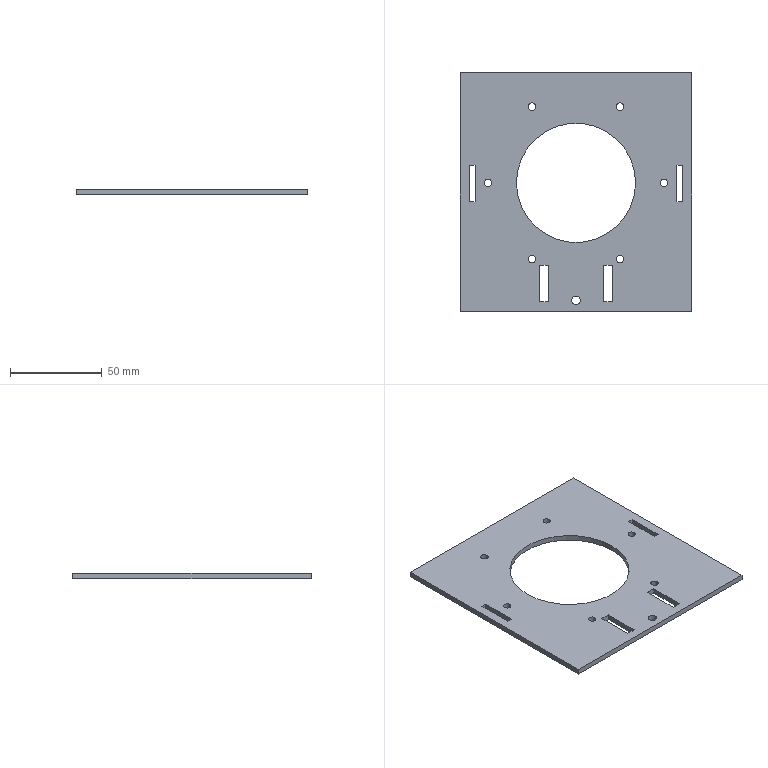Part | SolidWorks | features Cut 2, Extrusion 1, HoleWzd 1, MirrorPattern 1 | 1 solid | 38 faces | box 126 x 130 x 3 mm | volume 37973 mm3 | plane 22 | cylinder 16 | commonest cylinder face diameters 4 x12 4.6 x2 65 x2
STEP:
#1=CARTESIAN_POINT('',(-2.3,-64.,0.));
#2=VERTEX_POINT('',#1);
#3=CARTESIAN_POINT('',(2.3,-64.,0.));
#4=VERTEX_POINT('',#3);
#5=CARTESIAN_POINT('',(0.,-64.,0.));
#6=DIRECTION('',(0.,0.,1.));
#7=DIRECTION('',(1.,0.,0.));
#8=AXIS2_PLACEMENT_3D('',#5,#6,#7);
#9=CIRCLE('',#8,2.3);
#10=EDGE_CURVE('',#2,#4,#9,.T.);
#11=ORIENTED_EDGE('',*,*,#10,.F.);
#12=CARTESIAN_POINT('',(-2.3,-64.,3.));
#13=VERTEX_POINT('',#12);
#14=CARTESIAN_POINT('',(-2.3,-64.,0.));
#15=DIRECTION('',(0.,0.,1.));
#16=VECTOR('',#15,1000.);
#17=LINE('',#14,#16);
#18=EDGE_CURVE('',#2,#13,#17,.T.);
#19=ORIENTED_EDGE('',*,*,#18,.T.);
#20=CARTESIAN_POINT('',(2.3,-64.,3.));
#21=VERTEX_POINT('',#20);
#22=CARTESIAN_POINT('',(0.,-64.,3.));
#23=DIRECTION('',(0.,0.,1.));
#24=DIRECTION('',(1.,0.,0.));
#25=AXIS2_PLACEMENT_3D('',#22,#23,#24);
#26=CIRCLE('',#25,2.3);
#27=EDGE_CURVE('',#13,#21,#26,.T.);
#28=ORIENTED_EDGE('',*,*,#27,.T.);
#29=CARTESIAN_POINT('',(2.3,-64.,0.));
#30=DIRECTION('',(0.,0.,1.));
#31=VECTOR('',#30,1000.);
#32=LINE('',#29,#31);
#33=EDGE_CURVE('',#4,#21,#32,.T.);
#34=ORIENTED_EDGE('',*,*,#33,.F.);
#35=EDGE_LOOP('',(#11,#19,#28,#34));
#36=FACE_OUTER_BOUND('',#35,.T.);
#37=CARTESIAN_POINT('',(0.,-64.,0.));
#38=DIRECTION('',(0.,0.,1.));
#39=DIRECTION('',(1.,0.,0.));
#40=AXIS2_PLACEMENT_3D('',#37,#38,#39);
#41=CYLINDRICAL_SURFACE('',#40,2.3);
#42=ADVANCED_FACE('',(#36),#41,.F.);
#43=CARTESIAN_POINT('',(-26.,41.569,0.));
#44=VERTEX_POINT('',#43);
#45=CARTESIAN_POINT('',(-22.,41.569,0.));
#46=VERTEX_POINT('',#45);
#47=CARTESIAN_POINT('',(-24.,41.569,0.));
#48=DIRECTION('',(0.,0.,1.));
#49=DIRECTION('',(1.,0.,0.));
#50=AXIS2_PLACEMENT_3D('',#47,#48,#49);
#51=CIRCLE('',#50,2.);
#52=EDGE_CURVE('',#44,#46,#51,.T.);
#53=ORIENTED_EDGE('',*,*,#52,.F.);
#54=CARTESIAN_POINT('',(-26.,41.569,3.));
#55=VERTEX_POINT('',#54);
#56=CARTESIAN_POINT('',(-26.,41.569,3.));
#57=DIRECTION('',(0.,0.,1.));
#58=VECTOR('',#57,1000.);
#59=LINE('',#56,#58);
#60=EDGE_CURVE('',#44,#55,#59,.T.);
#61=ORIENTED_EDGE('',*,*,#60,.T.);
#62=CARTESIAN_POINT('',(-22.,41.569,3.));
#63=VERTEX_POINT('',#62);
#64=CARTESIAN_POINT('',(-24.,41.569,3.));
#65=DIRECTION('',(0.,0.,1.));
#66=DIRECTION('',(1.,0.,0.));
#67=AXIS2_PLACEMENT_3D('',#64,#65,#66);
#68=CIRCLE('',#67,2.);
#69=EDGE_CURVE('',#55,#63,#68,.T.);
#70=ORIENTED_EDGE('',*,*,#69,.T.);
#71=CARTESIAN_POINT('',(-22.,41.569,3.));
#72=DIRECTION('',(0.,0.,1.));
#73=VECTOR('',#72,1000.);
#74=LINE('',#71,#73);
#75=EDGE_CURVE('',#46,#63,#74,.T.);
#76=ORIENTED_EDGE('',*,*,#75,.F.);
#77=EDGE_LOOP('',(#53,#61,#70,#76));
#78=FACE_OUTER_BOUND('',#77,.T.);
#79=CARTESIAN_POINT('',(-24.,41.569,3.));
#80=DIRECTION('',(0.,0.,1.));
#81=DIRECTION('',(1.,0.,0.));
#82=AXIS2_PLACEMENT_3D('',#79,#80,#81);
#83=CYLINDRICAL_SURFACE('',#82,2.);
#84=ADVANCED_FACE('',(#78),#83,.F.);
#85=CARTESIAN_POINT('',(46.,0.,0.));
#86=VERTEX_POINT('',#85);
#87=CARTESIAN_POINT('',(50.,0.,0.));
#88=VERTEX_POINT('',#87);
#89=CARTESIAN_POINT('',(48.,0.,0.));
#90=DIRECTION('',(0.,0.,1.));
#91=DIRECTION('',(1.,0.,0.));
#92=AXIS2_PLACEMENT_3D('',#89,#90,#91);
#93=CIRCLE('',#92,2.);
#94=EDGE_CURVE('',#86,#88,#93,.T.);
#95=ORIENTED_EDGE('',*,*,#94,.F.);
#96=CARTESIAN_POINT('',(46.,0.,3.));
#97=VERTEX_POINT('',#96);
#98=CARTESIAN_POINT('',(46.,0.,3.));
#99=DIRECTION('',(0.,0.,1.));
#100=VECTOR('',#99,1000.);
#101=LINE('',#98,#100);
#102=EDGE_CURVE('',#86,#97,#101,.T.);
#103=ORIENTED_EDGE('',*,*,#102,.T.);
#104=CARTESIAN_POINT('',(50.,0.,3.));
#105=VERTEX_POINT('',#104);
#106=CARTESIAN_POINT('',(48.,0.,3.));
#107=DIRECTION('',(0.,0.,1.));
#108=DIRECTION('',(1.,0.,0.));
#109=AXIS2_PLACEMENT_3D('',#106,#107,#108);
#110=CIRCLE('',#109,2.);
#111=EDGE_CURVE('',#97,#105,#110,.T.);
#112=ORIENTED_EDGE('',*,*,#111,.T.);
#113=CARTESIAN_POINT('',(50.,0.,3.));
#114=DIRECTION('',(0.,0.,1.));
#115=VECTOR('',#114,1000.);
#116=LINE('',#113,#115);
#117=EDGE_CURVE('',#88,#105,#116,.T.);
#118=ORIENTED_EDGE('',*,*,#117,.F.);
#119=EDGE_LOOP('',(#95,#103,#112,#118));
#120=FACE_OUTER_BOUND('',#119,.T.);
#121=CARTESIAN_POINT('',(48.,0.,3.));
#122=DIRECTION('',(0.,0.,1.));
#123=DIRECTION('',(1.,0.,0.));
#124=AXIS2_PLACEMENT_3D('',#121,#122,#123);
#125=CYLINDRICAL_SURFACE('',#124,2.);
#126=ADVANCED_FACE('',(#120),#125,.F.);
#127=CARTESIAN_POINT('',(22.,41.569,0.));
#128=VERTEX_POINT('',#127);
#129=CARTESIAN_POINT('',(26.,41.569,0.));
#130=VERTEX_POINT('',#129);
#131=CARTESIAN_POINT('',(24.,41.569,0.));
#132=DIRECTION('',(0.,0.,1.));
#133=DIRECTION('',(1.,0.,0.));
#134=AXIS2_PLACEMENT_3D('',#131,#132,#133);
#135=CIRCLE('',#134,2.);
#136=EDGE_CURVE('',#128,#130,#135,.T.);
#137=ORIENTED_EDGE('',*,*,#136,.F.);
#138=CARTESIAN_POINT('',(22.,41.569,3.));
#139=VERTEX_POINT('',#138);
#140=CARTESIAN_POINT('',(22.,41.569,3.));
#141=DIRECTION('',(0.,0.,1.));
#142=VECTOR('',#141,1000.);
#143=LINE('',#140,#142);
#144=EDGE_CURVE('',#128,#139,#143,.T.);
#145=ORIENTED_EDGE('',*,*,#144,.T.);
#146=CARTESIAN_POINT('',(26.,41.569,3.));
#147=VERTEX_POINT('',#146);
#148=CARTESIAN_POINT('',(24.,41.569,3.));
#149=DIRECTION('',(0.,0.,1.));
#150=DIRECTION('',(1.,0.,0.));
#151=AXIS2_PLACEMENT_3D('',#148,#149,#150);
#152=CIRCLE('',#151,2.);
#153=EDGE_CURVE('',#139,#147,#152,.T.);
#154=ORIENTED_EDGE('',*,*,#153,.T.);
#155=CARTESIAN_POINT('',(26.,41.569,3.));
#156=DIRECTION('',(0.,0.,1.));
#157=VECTOR('',#156,1000.);
#158=LINE('',#155,#157);
#159=EDGE_CURVE('',#130,#147,#158,.T.);
#160=ORIENTED_EDGE('',*,*,#159,.F.);
#161=EDGE_LOOP('',(#137,#145,#154,#160));
#162=FACE_OUTER_BOUND('',#161,.T.);
#163=CARTESIAN_POINT('',(24.,41.569,3.));
#164=DIRECTION('',(0.,0.,1.));
#165=DIRECTION('',(1.,0.,0.));
#166=AXIS2_PLACEMENT_3D('',#163,#164,#165);
#167=CYLINDRICAL_SURFACE('',#166,2.);
#168=ADVANCED_FACE('',(#162),#167,.F.);
#169=CARTESIAN_POINT('',(22.,-41.569,0.));
#170=VERTEX_POINT('',#169);
#171=CARTESIAN_POINT('',(26.,-41.569,0.));
#172=VERTEX_POINT('',#171);
#173=CARTESIAN_POINT('',(24.,-41.569,0.));
#174=DIRECTION('',(0.,0.,1.));
#175=DIRECTION('',(1.,0.,0.));
#176=AXIS2_PLACEMENT_3D('',#173,#174,#175);
#177=CIRCLE('',#176,2.);
#178=EDGE_CURVE('',#170,#172,#177,.T.);
#179=ORIENTED_EDGE('',*,*,#178,.F.);
#180=CARTESIAN_POINT('',(22.,-41.569,3.));
#181=VERTEX_POINT('',#180);
#182=CARTESIAN_POINT('',(22.,-41.569,3.));
#183=DIRECTION('',(0.,0.,1.));
#184=VECTOR('',#183,1000.);
#185=LINE('',#182,#184);
#186=EDGE_CURVE('',#170,#181,#185,.T.);
#187=ORIENTED_EDGE('',*,*,#186,.T.);
#188=CARTESIAN_POINT('',(26.,-41.569,3.));
#189=VERTEX_POINT('',#188);
#190=CARTESIAN_POINT('',(24.,-41.569,3.));
#191=DIRECTION('',(0.,0.,1.));
#192=DIRECTION('',(1.,0.,0.));
#193=AXIS2_PLACEMENT_3D('',#190,#191,#192);
#194=CIRCLE('',#193,2.);
#195=EDGE_CURVE('',#181,#189,#194,.T.);
#196=ORIENTED_EDGE('',*,*,#195,.T.);
#197=CARTESIAN_POINT('',(26.,-41.569,3.));
#198=DIRECTION('',(0.,0.,1.));
#199=VECTOR('',#198,1000.);
#200=LINE('',#197,#199);
#201=EDGE_CURVE('',#172,#189,#200,.T.);
#202=ORIENTED_EDGE('',*,*,#201,.F.);
#203=EDGE_LOOP('',(#179,#187,#196,#202));
#204=FACE_OUTER_BOUND('',#203,.T.);
#205=CARTESIAN_POINT('',(24.,-41.569,3.));
#206=DIRECTION('',(0.,0.,1.));
#207=DIRECTION('',(1.,0.,0.));
#208=AXIS2_PLACEMENT_3D('',#205,#206,#207);
#209=CYLINDRICAL_SURFACE('',#208,2.);
#210=ADVANCED_FACE('',(#204),#209,.F.);
#211=CARTESIAN_POINT('',(-26.,-41.569,0.));
#212=VERTEX_POINT('',#211);
#213=CARTESIAN_POINT('',(-22.,-41.569,0.));
#214=VERTEX_POINT('',#213);
#215=CARTESIAN_POINT('',(-24.,-41.569,0.));
#216=DIRECTION('',(0.,0.,1.));
#217=DIRECTION('',(1.,0.,0.));
#218=AXIS2_PLACEMENT_3D('',#215,#216,#217);
#219=CIRCLE('',#218,2.);
#220=EDGE_CURVE('',#212,#214,#219,.T.);
#221=ORIENTED_EDGE('',*,*,#220,.F.);
#222=CARTESIAN_POINT('',(-26.,-41.569,3.));
#223=VERTEX_POINT('',#222);
#224=CARTESIAN_POINT('',(-26.,-41.569,3.));
#225=DIRECTION('',(0.,0.,1.));
#226=VECTOR('',#225,1000.);
#227=LINE('',#224,#226);
#228=EDGE_CURVE('',#212,#223,#227,.T.);
#229=ORIENTED_EDGE('',*,*,#228,.T.);
#230=CARTESIAN_POINT('',(-22.,-41.569,3.));
#231=VERTEX_POINT('',#230);
#232=CARTESIAN_POINT('',(-24.,-41.569,3.));
#233=DIRECTION('',(0.,0.,1.));
#234=DIRECTION('',(1.,0.,0.));
#235=AXIS2_PLACEMENT_3D('',#232,#233,#234);
#236=CIRCLE('',#235,2.);
#237=EDGE_CURVE('',#223,#231,#236,.T.);
#238=ORIENTED_EDGE('',*,*,#237,.T.);
#239=CARTESIAN_POINT('',(-22.,-41.569,3.));
#240=DIRECTION('',(0.,0.,1.));
#241=VECTOR('',#240,1000.);
#242=LINE('',#239,#241);
#243=EDGE_CURVE('',#214,#231,#242,.T.);
#244=ORIENTED_EDGE('',*,*,#243,.F.);
#245=EDGE_LOOP('',(#221,#229,#238,#244));
#246=FACE_OUTER_BOUND('',#245,.T.);
#247=CARTESIAN_POINT('',(-24.,-41.569,3.));
#248=DIRECTION('',(0.,0.,1.));
#249=DIRECTION('',(1.,0.,0.));
#250=AXIS2_PLACEMENT_3D('',#247,#248,#249);
#251=CYLINDRICAL_SURFACE('',#250,2.);
#252=ADVANCED_FACE('',(#246),#251,.F.);
#253=CARTESIAN_POINT('',(-50.,0.,0.));
#254=VERTEX_POINT('',#253);
#255=CARTESIAN_POINT('',(-46.,0.,0.));
#256=VERTEX_POINT('',#255);
#257=CARTESIAN_POINT('',(-48.,0.,0.));
#258=DIRECTION('',(0.,0.,1.));
#259=DIRECTION('',(1.,0.,0.));
#260=AXIS2_PLACEMENT_3D('',#257,#258,#259);
#261=CIRCLE('',#260,2.);
#262=EDGE_CURVE('',#254,#256,#261,.T.);
#263=ORIENTED_EDGE('',*,*,#262,.F.);
#264=CARTESIAN_POINT('',(-50.,0.,3.));
#265=VERTEX_POINT('',#264);
#266=CARTESIAN_POINT('',(-50.,0.,3.));
#267=DIRECTION('',(0.,0.,1.));
#268=VECTOR('',#267,1000.);
#269=LINE('',#266,#268);
#270=EDGE_CURVE('',#254,#265,#269,.T.);
#271=ORIENTED_EDGE('',*,*,#270,.T.);
#272=CARTESIAN_POINT('',(-46.,0.,3.));
#273=VERTEX_POINT('',#272);
#274=CARTESIAN_POINT('',(-48.,0.,3.));
#275=DIRECTION('',(0.,0.,1.));
#276=DIRECTION('',(1.,0.,0.));
#277=AXIS2_PLACEMENT_3D('',#274,#275,#276);
#278=CIRCLE('',#277,2.);
#279=EDGE_CURVE('',#265,#273,#278,.T.);
#280=ORIENTED_EDGE('',*,*,#279,.T.);
#281=CARTESIAN_POINT('',(-46.,0.,3.));
#282=DIRECTION('',(0.,0.,1.));
#283=VECTOR('',#282,1000.);
#284=LINE('',#281,#283);
#285=EDGE_CURVE('',#256,#273,#284,.T.);
#286=ORIENTED_EDGE('',*,*,#285,.F.);
#287=EDGE_LOOP('',(#263,#271,#280,#286));
#288=FACE_OUTER_BOUND('',#287,.T.);
#289=CARTESIAN_POINT('',(-48.,0.,3.));
#290=DIRECTION('',(0.,0.,1.));
#291=DIRECTION('',(1.,0.,0.));
#292=AXIS2_PLACEMENT_3D('',#289,#290,#291);
#293=CYLINDRICAL_SURFACE('',#292,2.);
#294=ADVANCED_FACE('',(#288),#293,.F.);
#295=CARTESIAN_POINT('',(-32.5,0.,3.));
#296=VERTEX_POINT('',#295);
#297=CARTESIAN_POINT('',(32.5,0.,3.));
#298=VERTEX_POINT('',#297);
#299=CARTESIAN_POINT('',(0.,0.,3.));
#300=DIRECTION('',(0.,0.,1.));
#301=DIRECTION('',(1.,0.,0.));
#302=AXIS2_PLACEMENT_3D('',#299,#300,#301);
#303=CIRCLE('',#302,32.5);
#304=EDGE_CURVE('',#296,#298,#303,.T.);
#305=ORIENTED_EDGE('',*,*,#304,.T.);
#306=CARTESIAN_POINT('',(32.5,0.,0.));
#307=VERTEX_POINT('',#306);
#308=CARTESIAN_POINT('',(32.5,0.,3.));
#309=DIRECTION('',(0.,0.,-1.));
#310=VECTOR('',#309,1000.);
#311=LINE('',#308,#310);
#312=EDGE_CURVE('',#298,#307,#311,.T.);
#313=ORIENTED_EDGE('',*,*,#312,.T.);
#314=CARTESIAN_POINT('',(-32.5,0.,0.));
#315=VERTEX_POINT('',#314);
#316=CARTESIAN_POINT('',(0.,0.,0.));
#317=DIRECTION('',(0.,0.,1.));
#318=DIRECTION('',(1.,0.,0.));
#319=AXIS2_PLACEMENT_3D('',#316,#317,#318);
#320=CIRCLE('',#319,32.5);
#321=EDGE_CURVE('',#315,#307,#320,.T.);
#322=ORIENTED_EDGE('',*,*,#321,.F.);
#323=CARTESIAN_POINT('',(-32.5,0.,3.));
#324=DIRECTION('',(0.,0.,-1.));
#325=VECTOR('',#324,1000.);
#326=LINE('',#323,#325);
#327=EDGE_CURVE('',#296,#315,#326,.T.);
#328=ORIENTED_EDGE('',*,*,#327,.F.);
#329=EDGE_LOOP('',(#305,#313,#322,#328));
#330=FACE_OUTER_BOUND('',#329,.T.);
#331=CARTESIAN_POINT('',(0.,0.,3.));
#332=DIRECTION('',(0.,0.,-1.));
#333=DIRECTION('',(-1.,0.,0.));
#334=AXIS2_PLACEMENT_3D('',#331,#332,#333);
#335=CYLINDRICAL_SURFACE('',#334,32.5);
#336=ADVANCED_FACE('',(#330),#335,.F.);
#337=CARTESIAN_POINT('',(0.,-64.,3.));
#338=DIRECTION('',(0.,0.,1.));
#339=DIRECTION('',(1.,0.,0.));
#340=AXIS2_PLACEMENT_3D('',#337,#338,#339);
#341=CIRCLE('',#340,2.3);
#342=EDGE_CURVE('',#21,#13,#341,.T.);
#343=ORIENTED_EDGE('',*,*,#342,.F.);
#344=ORIENTED_EDGE('',*,*,#27,.F.);
#345=EDGE_LOOP('',(#343,#344));
#346=FACE_BOUND('',#345,.T.);
#347=CARTESIAN_POINT('',(-24.,41.569,3.));
#348=DIRECTION('',(0.,0.,1.));
#349=DIRECTION('',(1.,0.,0.));
#350=AXIS2_PLACEMENT_3D('',#347,#348,#349);
#351=CIRCLE('',#350,2.);
#352=EDGE_CURVE('',#63,#55,#351,.T.);
#353=ORIENTED_EDGE('',*,*,#352,.F.);
#354=ORIENTED_EDGE('',*,*,#69,.F.);
#355=EDGE_LOOP('',(#353,#354));
#356=FACE_BOUND('',#355,.T.);
#357=CARTESIAN_POINT('',(48.,0.,3.));
#358=DIRECTION('',(0.,0.,1.));
#359=DIRECTION('',(1.,0.,0.));
#360=AXIS2_PLACEMENT_3D('',#357,#358,#359);
#361=CIRCLE('',#360,2.);
#362=EDGE_CURVE('',#105,#97,#361,.T.);
#363=ORIENTED_EDGE('',*,*,#362,.F.);
#364=ORIENTED_EDGE('',*,*,#111,.F.);
#365=EDGE_LOOP('',(#363,#364));
#366=FACE_BOUND('',#365,.T.);
#367=CARTESIAN_POINT('',(24.,41.569,3.));
#368=DIRECTION('',(0.,0.,1.));
#369=DIRECTION('',(1.,0.,0.));
#370=AXIS2_PLACEMENT_3D('',#367,#368,#369);
#371=CIRCLE('',#370,2.);
#372=EDGE_CURVE('',#147,#139,#371,.T.);
#373=ORIENTED_EDGE('',*,*,#372,.F.);
#374=ORIENTED_EDGE('',*,*,#153,.F.);
#375=EDGE_LOOP('',(#373,#374));
#376=FACE_BOUND('',#375,.T.);
#377=CARTESIAN_POINT('',(24.,-41.569,3.));
#378=DIRECTION('',(0.,0.,1.));
#379=DIRECTION('',(1.,0.,0.));
#380=AXIS2_PLACEMENT_3D('',#377,#378,#379);
#381=CIRCLE('',#380,2.);
#382=EDGE_CURVE('',#189,#181,#381,.T.);
#383=ORIENTED_EDGE('',*,*,#382,.F.);
#384=ORIENTED_EDGE('',*,*,#195,.F.);
#385=EDGE_LOOP('',(#383,#384));
#386=FACE_BOUND('',#385,.T.);
#387=CARTESIAN_POINT('',(-24.,-41.569,3.));
#388=DIRECTION('',(0.,0.,1.));
#389=DIRECTION('',(1.,0.,0.));
#390=AXIS2_PLACEMENT_3D('',#387,#388,#389);
#391=CIRCLE('',#390,2.);
#392=EDGE_CURVE('',#231,#223,#391,.T.);
#393=ORIENTED_EDGE('',*,*,#392,.F.);
#394=ORIENTED_EDGE('',*,*,#237,.F.);
#395=EDGE_LOOP('',(#393,#394));
#396=FACE_BOUND('',#395,.T.);
#397=CARTESIAN_POINT('',(-48.,0.,3.));
#398=DIRECTION('',(0.,0.,1.));
#399=DIRECTION('',(1.,0.,0.));
#400=AXIS2_PLACEMENT_3D('',#397,#398,#399);
#401=CIRCLE('',#400,2.);
#402=EDGE_CURVE('',#273,#265,#401,.T.);
#403=ORIENTED_EDGE('',*,*,#402,.F.);
#404=ORIENTED_EDGE('',*,*,#279,.F.);
#405=EDGE_LOOP('',(#403,#404));
#406=FACE_BOUND('',#405,.T.);
#407=CARTESIAN_POINT('',(15.05,-44.9,3.));
#408=VERTEX_POINT('',#407);
#409=CARTESIAN_POINT('',(15.05,-64.9,3.));
#410=VERTEX_POINT('',#409);
#411=CARTESIAN_POINT('',(15.05,-44.9,3.));
#412=DIRECTION('',(0.,-1.,0.));
#413=VECTOR('',#412,1000.);
#414=LINE('',#411,#413);
#415=EDGE_CURVE('',#408,#410,#414,.T.);
#416=ORIENTED_EDGE('',*,*,#415,.F.);
#417=CARTESIAN_POINT('',(19.95,-44.9,3.));
#418=VERTEX_POINT('',#417);
#419=CARTESIAN_POINT('',(19.95,-44.9,3.));
#420=DIRECTION('',(-1.,0.,0.));
#421=VECTOR('',#420,1000.);
#422=LINE('',#419,#421);
#423=EDGE_CURVE('',#418,#408,#422,.T.);
#424=ORIENTED_EDGE('',*,*,#423,.F.);
#425=CARTESIAN_POINT('',(19.95,-64.9,3.));
#426=VERTEX_POINT('',#425);
#427=CARTESIAN_POINT('',(19.95,-44.9,3.));
#428=DIRECTION('',(0.,1.,0.));
#429=VECTOR('',#428,1000.);
#430=LINE('',#427,#429);
#431=EDGE_CURVE('',#426,#418,#430,.T.);
#432=ORIENTED_EDGE('',*,*,#431,.F.);
#433=CARTESIAN_POINT('',(19.95,-64.9,3.));
#434=DIRECTION('',(1.,0.,0.));
#435=VECTOR('',#434,1000.);
#436=LINE('',#433,#435);
#437=EDGE_CURVE('',#410,#426,#436,.T.);
#438=ORIENTED_EDGE('',*,*,#437,.F.);
#439=EDGE_LOOP('',(#416,#424,#432,#438));
#440=FACE_BOUND('',#439,.T.);
#441=ORIENTED_EDGE('',*,*,#304,.F.);
#442=CARTESIAN_POINT('',(0.,0.,3.));
#443=DIRECTION('',(0.,0.,1.));
#444=DIRECTION('',(1.,0.,0.));
#445=AXIS2_PLACEMENT_3D('',#442,#443,#444);
#446=CIRCLE('',#445,32.5);
#447=EDGE_CURVE('',#298,#296,#446,.T.);
#448=ORIENTED_EDGE('',*,*,#447,.F.);
#449=EDGE_LOOP('',(#441,#448));
#450=FACE_BOUND('',#449,.T.);
#451=CARTESIAN_POINT('',(-63.,60.,3.));
#452=VERTEX_POINT('',#451);
#453=CARTESIAN_POINT('',(-63.,-70.,3.));
#454=VERTEX_POINT('',#453);
#455=CARTESIAN_POINT('',(-63.,60.,3.));
#456=DIRECTION('',(0.,-1.,0.));
#457=VECTOR('',#456,1000.);
#458=LINE('',#455,#457);
#459=EDGE_CURVE('',#452,#454,#458,.T.);
#460=ORIENTED_EDGE('',*,*,#459,.T.);
#461=CARTESIAN_POINT('',(63.,-70.,3.));
#462=VERTEX_POINT('',#461);
#463=CARTESIAN_POINT('',(-63.,-70.,3.));
#464=DIRECTION('',(1.,0.,0.));
#465=VECTOR('',#464,1000.);
#466=LINE('',#463,#465);
#467=EDGE_CURVE('',#454,#462,#466,.T.);
#468=ORIENTED_EDGE('',*,*,#467,.T.);
#469=CARTESIAN_POINT('',(63.,60.,3.));
#470=VERTEX_POINT('',#469);
#471=CARTESIAN_POINT('',(63.,60.,3.));
#472=DIRECTION('',(0.,1.,0.));
#473=VECTOR('',#472,1000.);
#474=LINE('',#471,#473);
#475=EDGE_CURVE('',#462,#470,#474,.T.);
#476=ORIENTED_EDGE('',*,*,#475,.T.);
#477=CARTESIAN_POINT('',(-63.,60.,3.));
#478=DIRECTION('',(-1.,0.,0.));
#479=VECTOR('',#478,1000.);
#480=LINE('',#477,#479);
#481=EDGE_CURVE('',#470,#452,#480,.T.);
#482=ORIENTED_EDGE('',*,*,#481,.T.);
#483=EDGE_LOOP('',(#460,#468,#476,#482));
#484=FACE_OUTER_BOUND('',#483,.T.);
#485=CARTESIAN_POINT('',(-15.05,-44.9,3.));
#486=VERTEX_POINT('',#485);
#487=CARTESIAN_POINT('',(-19.95,-44.9,3.));
#488=VERTEX_POINT('',#487);
#489=CARTESIAN_POINT('',(-15.05,-44.9,3.));
#490=DIRECTION('',(-1.,0.,0.));
#491=VECTOR('',#490,1000.);
#492=LINE('',#489,#491);
#493=EDGE_CURVE('',#486,#488,#492,.T.);
#494=ORIENTED_EDGE('',*,*,#493,.F.);
#495=CARTESIAN_POINT('',(-15.05,-64.9,3.));
#496=VERTEX_POINT('',#495);
#497=CARTESIAN_POINT('',(-15.05,-44.9,3.));
#498=DIRECTION('',(0.,1.,0.));
#499=VECTOR('',#498,1000.);
#500=LINE('',#497,#499);
#501=EDGE_CURVE('',#496,#486,#500,.T.);
#502=ORIENTED_EDGE('',*,*,#501,.F.);
#503=CARTESIAN_POINT('',(-19.95,-64.9,3.));
#504=VERTEX_POINT('',#503);
#505=CARTESIAN_POINT('',(-15.05,-64.9,3.));
#506=DIRECTION('',(1.,0.,0.));
#507=VECTOR('',#506,1000.);
#508=LINE('',#505,#507);
#509=EDGE_CURVE('',#504,#496,#508,.T.);
#510=ORIENTED_EDGE('',*,*,#509,.F.);
#511=CARTESIAN_POINT('',(-19.95,-44.9,3.));
#512=DIRECTION('',(0.,-1.,0.));
#513=VECTOR('',#512,1000.);
#514=LINE('',#511,#513);
#515=EDGE_CURVE('',#488,#504,#514,.T.);
#516=ORIENTED_EDGE('',*,*,#515,.F.);
#517=EDGE_LOOP('',(#494,#502,#510,#516));
#518=FACE_BOUND('',#517,.T.);
#519=CARTESIAN_POINT('',(-57.95,9.6,3.));
#520=VERTEX_POINT('',#519);
#521=CARTESIAN_POINT('',(-57.95,-10.4,3.));
#522=VERTEX_POINT('',#521);
#523=CARTESIAN_POINT('',(-57.95,9.6,3.));
#524=DIRECTION('',(0.,-1.,0.));
#525=VECTOR('',#524,1000.);
#526=LINE('',#523,#525);
#527=EDGE_CURVE('',#520,#522,#526,.T.);
#528=ORIENTED_EDGE('',*,*,#527,.F.);
#529=CARTESIAN_POINT('',(-55.05,9.6,3.));
#530=VERTEX_POINT('',#529);
#531=CARTESIAN_POINT('',(-57.95,9.6,3.));
#532=DIRECTION('',(-1.,0.,0.));
#533=VECTOR('',#532,1000.);
#534=LINE('',#531,#533);
#535=EDGE_CURVE('',#530,#520,#534,.T.);
#536=ORIENTED_EDGE('',*,*,#535,.F.);
#537=CARTESIAN_POINT('',(-55.05,-10.4,3.));
#538=VERTEX_POINT('',#537);
#539=CARTESIAN_POINT('',(-55.05,9.6,3.));
#540=DIRECTION('',(0.,1.,0.));
#541=VECTOR('',#540,1000.);
#542=LINE('',#539,#541);
#543=EDGE_CURVE('',#538,#530,#542,.T.);
#544=ORIENTED_EDGE('',*,*,#543,.F.);
#545=CARTESIAN_POINT('',(-57.95,-10.4,3.));
#546=DIRECTION('',(1.,0.,0.));
#547=VECTOR('',#546,1000.);
#548=LINE('',#545,#547);
#549=EDGE_CURVE('',#522,#538,#548,.T.);
#550=ORIENTED_EDGE('',*,*,#549,.F.);
#551=EDGE_LOOP('',(#528,#536,#544,#550));
#552=FACE_BOUND('',#551,.T.);
#553=CARTESIAN_POINT('',(55.05,9.6,3.));
#554=VERTEX_POINT('',#553);
#555=CARTESIAN_POINT('',(57.95,9.6,3.));
#556=VERTEX_POINT('',#555);
#557=CARTESIAN_POINT('',(57.95,9.6,3.));
#558=DIRECTION('',(1.,0.,0.));
#559=VECTOR('',#558,1000.);
#560=LINE('',#557,#559);
#561=EDGE_CURVE('',#554,#556,#560,.T.);
#562=ORIENTED_EDGE('',*,*,#561,.T.);
#563=CARTESIAN_POINT('',(57.95,-10.4,3.));
#564=VERTEX_POINT('',#563);
#565=CARTESIAN_POINT('',(57.95,9.6,3.));
#566=DIRECTION('',(0.,-1.,0.));
#567=VECTOR('',#566,1000.);
#568=LINE('',#565,#567);
#569=EDGE_CURVE('',#556,#564,#568,.T.);
#570=ORIENTED_EDGE('',*,*,#569,.T.);
#571=CARTESIAN_POINT('',(55.05,-10.4,3.));
#572=VERTEX_POINT('',#571);
#573=CARTESIAN_POINT('',(57.95,-10.4,3.));
#574=DIRECTION('',(-1.,0.,0.));
#575=VECTOR('',#574,1000.);
#576=LINE('',#573,#575);
#577=EDGE_CURVE('',#564,#572,#576,.T.);
#578=ORIENTED_EDGE('',*,*,#577,.T.);
#579=CARTESIAN_POINT('',(55.05,9.6,3.));
#580=DIRECTION('',(0.,1.,0.));
#581=VECTOR('',#580,1000.);
#582=LINE('',#579,#581);
#583=EDGE_CURVE('',#572,#554,#582,.T.);
#584=ORIENTED_EDGE('',*,*,#583,.T.);
#585=EDGE_LOOP('',(#562,#570,#578,#584));
#586=FACE_BOUND('',#585,.T.);
#587=CARTESIAN_POINT('',(0.,0.,3.));
#588=DIRECTION('',(0.,0.,1.));
#589=DIRECTION('',(1.,0.,0.));
#590=AXIS2_PLACEMENT_3D('',#587,#588,#589);
#591=PLANE('',#590);
#592=ADVANCED_FACE('',(#346,#356,#366,#376,#386,#396,#406,#440,#450,#484,#518,#552,#586),#591,.T.);
#593=CARTESIAN_POINT('',(0.,-64.,0.));
#594=DIRECTION('',(0.,0.,1.));
#595=DIRECTION('',(1.,0.,0.));
#596=AXIS2_PLACEMENT_3D('',#593,#594,#595);
#597=CIRCLE('',#596,2.3);
#598=EDGE_CURVE('',#4,#2,#597,.T.);
#599=ORIENTED_EDGE('',*,*,#598,.T.);
#600=ORIENTED_EDGE('',*,*,#10,.T.);
#601=EDGE_LOOP('',(#599,#600));
#602=FACE_BOUND('',#601,.T.);
#603=CARTESIAN_POINT('',(-24.,41.569,0.));
#604=DIRECTION('',(0.,0.,1.));
#605=DIRECTION('',(1.,0.,0.));
#606=AXIS2_PLACEMENT_3D('',#603,#604,#605);
#607=CIRCLE('',#606,2.);
#608=EDGE_CURVE('',#46,#44,#607,.T.);
#609=ORIENTED_EDGE('',*,*,#608,.T.);
#610=ORIENTED_EDGE('',*,*,#52,.T.);
#611=EDGE_LOOP('',(#609,#610));
#612=FACE_BOUND('',#611,.T.);
#613=CARTESIAN_POINT('',(48.,0.,0.));
#614=DIRECTION('',(0.,0.,1.));
#615=DIRECTION('',(1.,0.,0.));
#616=AXIS2_PLACEMENT_3D('',#613,#614,#615);
#617=CIRCLE('',#616,2.);
#618=EDGE_CURVE('',#88,#86,#617,.T.);
#619=ORIENTED_EDGE('',*,*,#618,.T.);
#620=ORIENTED_EDGE('',*,*,#94,.T.);
#621=EDGE_LOOP('',(#619,#620));
#622=FACE_BOUND('',#621,.T.);
#623=CARTESIAN_POINT('',(24.,41.569,0.));
#624=DIRECTION('',(0.,0.,1.));
#625=DIRECTION('',(1.,0.,0.));
#626=AXIS2_PLACEMENT_3D('',#623,#624,#625);
#627=CIRCLE('',#626,2.);
#628=EDGE_CURVE('',#130,#128,#627,.T.);
#629=ORIENTED_EDGE('',*,*,#628,.T.);
#630=ORIENTED_EDGE('',*,*,#136,.T.);
#631=EDGE_LOOP('',(#629,#630));
#632=FACE_BOUND('',#631,.T.);
#633=CARTESIAN_POINT('',(24.,-41.569,0.));
#634=DIRECTION('',(0.,0.,1.));
#635=DIRECTION('',(1.,0.,0.));
#636=AXIS2_PLACEMENT_3D('',#633,#634,#635);
#637=CIRCLE('',#636,2.);
#638=EDGE_CURVE('',#172,#170,#637,.T.);
#639=ORIENTED_EDGE('',*,*,#638,.T.);
#640=ORIENTED_EDGE('',*,*,#178,.T.);
#641=EDGE_LOOP('',(#639,#640));
#642=FACE_BOUND('',#641,.T.);
#643=CARTESIAN_POINT('',(-24.,-41.569,0.));
#644=DIRECTION('',(0.,0.,1.));
#645=DIRECTION('',(1.,0.,0.));
#646=AXIS2_PLACEMENT_3D('',#643,#644,#645);
#647=CIRCLE('',#646,2.);
#648=EDGE_CURVE('',#214,#212,#647,.T.);
#649=ORIENTED_EDGE('',*,*,#648,.T.);
#650=ORIENTED_EDGE('',*,*,#220,.T.);
#651=EDGE_LOOP('',(#649,#650));
#652=FACE_BOUND('',#651,.T.);
#653=CARTESIAN_POINT('',(-48.,0.,0.));
#654=DIRECTION('',(0.,0.,1.));
#655=DIRECTION('',(1.,0.,0.));
#656=AXIS2_PLACEMENT_3D('',#653,#654,#655);
#657=CIRCLE('',#656,2.);
#658=EDGE_CURVE('',#256,#254,#657,.T.);
#659=ORIENTED_EDGE('',*,*,#658,.T.);
#660=ORIENTED_EDGE('',*,*,#262,.T.);
#661=EDGE_LOOP('',(#659,#660));
#662=FACE_BOUND('',#661,.T.);
#663=CARTESIAN_POINT('',(19.95,-44.9,0.));
#664=VERTEX_POINT('',#663);
#665=CARTESIAN_POINT('',(15.05,-44.9,0.));
#666=VERTEX_POINT('',#665);
#667=CARTESIAN_POINT('',(19.95,-44.9,0.));
#668=DIRECTION('',(-1.,0.,0.));
#669=VECTOR('',#668,1000.);
#670=LINE('',#667,#669);
#671=EDGE_CURVE('',#664,#666,#670,.T.);
#672=ORIENTED_EDGE('',*,*,#671,.T.);
#673=CARTESIAN_POINT('',(15.05,-64.9,0.));
#674=VERTEX_POINT('',#673);
#675=CARTESIAN_POINT('',(15.05,-44.9,0.));
#676=DIRECTION('',(0.,-1.,0.));
#677=VECTOR('',#676,1000.);
#678=LINE('',#675,#677);
#679=EDGE_CURVE('',#666,#674,#678,.T.);
#680=ORIENTED_EDGE('',*,*,#679,.T.);
#681=CARTESIAN_POINT('',(19.95,-64.9,0.));
#682=VERTEX_POINT('',#681);
#683=CARTESIAN_POINT('',(19.95,-64.9,0.));
#684=DIRECTION('',(1.,0.,0.));
#685=VECTOR('',#684,1000.);
#686=LINE('',#683,#685);
#687=EDGE_CURVE('',#674,#682,#686,.T.);
#688=ORIENTED_EDGE('',*,*,#687,.T.);
#689=CARTESIAN_POINT('',(19.95,-44.9,0.));
#690=DIRECTION('',(0.,1.,0.));
#691=VECTOR('',#690,1000.);
#692=LINE('',#689,#691);
#693=EDGE_CURVE('',#682,#664,#692,.T.);
#694=ORIENTED_EDGE('',*,*,#693,.T.);
#695=EDGE_LOOP('',(#672,#680,#688,#694));
#696=FACE_BOUND('',#695,.T.);
#697=ORIENTED_EDGE('',*,*,#321,.T.);
#698=CARTESIAN_POINT('',(0.,0.,0.));
#699=DIRECTION('',(0.,0.,1.));
#700=DIRECTION('',(1.,0.,0.));
#701=AXIS2_PLACEMENT_3D('',#698,#699,#700);
#702=CIRCLE('',#701,32.5);
#703=EDGE_CURVE('',#307,#315,#702,.T.);
#704=ORIENTED_EDGE('',*,*,#703,.T.);
#705=EDGE_LOOP('',(#697,#704));
#706=FACE_BOUND('',#705,.T.);
#707=CARTESIAN_POINT('',(-63.,60.,0.));
#708=VERTEX_POINT('',#707);
#709=CARTESIAN_POINT('',(-63.,-70.,0.));
#710=VERTEX_POINT('',#709);
#711=CARTESIAN_POINT('',(-63.,60.,0.));
#712=DIRECTION('',(0.,-1.,0.));
#713=VECTOR('',#712,1000.);
#714=LINE('',#711,#713);
#715=EDGE_CURVE('',#708,#710,#714,.T.);
#716=ORIENTED_EDGE('',*,*,#715,.F.);
#717=CARTESIAN_POINT('',(63.,60.,0.));
#718=VERTEX_POINT('',#717);
#719=CARTESIAN_POINT('',(-63.,60.,0.));
#720=DIRECTION('',(-1.,0.,0.));
#721=VECTOR('',#720,1000.);
#722=LINE('',#719,#721);
#723=EDGE_CURVE('',#718,#708,#722,.T.);
#724=ORIENTED_EDGE('',*,*,#723,.F.);
#725=CARTESIAN_POINT('',(63.,-70.,0.));
#726=VERTEX_POINT('',#725);
#727=CARTESIAN_POINT('',(63.,60.,0.));
#728=DIRECTION('',(0.,1.,0.));
#729=VECTOR('',#728,1000.);
#730=LINE('',#727,#729);
#731=EDGE_CURVE('',#726,#718,#730,.T.);
#732=ORIENTED_EDGE('',*,*,#731,.F.);
#733=CARTESIAN_POINT('',(-63.,-70.,0.));
#734=DIRECTION('',(1.,0.,0.));
#735=VECTOR('',#734,1000.);
#736=LINE('',#733,#735);
#737=EDGE_CURVE('',#710,#726,#736,.T.);
#738=ORIENTED_EDGE('',*,*,#737,.F.);
#739=EDGE_LOOP('',(#716,#724,#732,#738));
#740=FACE_OUTER_BOUND('',#739,.T.);
#741=CARTESIAN_POINT('',(-15.05,-64.9,0.));
#742=VERTEX_POINT('',#741);
#743=CARTESIAN_POINT('',(-15.05,-44.9,0.));
#744=VERTEX_POINT('',#743);
#745=CARTESIAN_POINT('',(-15.05,-44.9,0.));
#746=DIRECTION('',(0.,1.,0.));
#747=VECTOR('',#746,1000.);
#748=LINE('',#745,#747);
#749=EDGE_CURVE('',#742,#744,#748,.T.);
#750=ORIENTED_EDGE('',*,*,#749,.T.);
#751=CARTESIAN_POINT('',(-19.95,-44.9,0.));
#752=VERTEX_POINT('',#751);
#753=CARTESIAN_POINT('',(-15.05,-44.9,0.));
#754=DIRECTION('',(-1.,0.,0.));
#755=VECTOR('',#754,1000.);
#756=LINE('',#753,#755);
#757=EDGE_CURVE('',#744,#752,#756,.T.);
#758=ORIENTED_EDGE('',*,*,#757,.T.);
#759=CARTESIAN_POINT('',(-19.95,-64.9,0.));
#760=VERTEX_POINT('',#759);
#761=CARTESIAN_POINT('',(-19.95,-44.9,0.));
#762=DIRECTION('',(0.,-1.,0.));
#763=VECTOR('',#762,1000.);
#764=LINE('',#761,#763);
#765=EDGE_CURVE('',#752,#760,#764,.T.);
#766=ORIENTED_EDGE('',*,*,#765,.T.);
#767=CARTESIAN_POINT('',(-15.05,-64.9,0.));
#768=DIRECTION('',(1.,0.,0.));
#769=VECTOR('',#768,1000.);
#770=LINE('',#767,#769);
#771=EDGE_CURVE('',#760,#742,#770,.T.);
#772=ORIENTED_EDGE('',*,*,#771,.T.);
#773=EDGE_LOOP('',(#750,#758,#766,#772));
#774=FACE_BOUND('',#773,.T.);
#775=CARTESIAN_POINT('',(-55.05,9.6,0.));
#776=VERTEX_POINT('',#775);
#777=CARTESIAN_POINT('',(-57.95,9.6,0.));
#778=VERTEX_POINT('',#777);
#779=CARTESIAN_POINT('',(-57.95,9.6,0.));
#780=DIRECTION('',(-1.,0.,0.));
#781=VECTOR('',#780,1000.);
#782=LINE('',#779,#781);
#783=EDGE_CURVE('',#776,#778,#782,.T.);
#784=ORIENTED_EDGE('',*,*,#783,.T.);
#785=CARTESIAN_POINT('',(-57.95,-10.4,0.));
#786=VERTEX_POINT('',#785);
#787=CARTESIAN_POINT('',(-57.95,9.6,0.));
#788=DIRECTION('',(0.,-1.,0.));
#789=VECTOR('',#788,1000.);
#790=LINE('',#787,#789);
#791=EDGE_CURVE('',#778,#786,#790,.T.);
#792=ORIENTED_EDGE('',*,*,#791,.T.);
#793=CARTESIAN_POINT('',(-55.05,-10.4,0.));
#794=VERTEX_POINT('',#793);
#795=CARTESIAN_POINT('',(-57.95,-10.4,0.));
#796=DIRECTION('',(1.,0.,0.));
#797=VECTOR('',#796,1000.);
#798=LINE('',#795,#797);
#799=EDGE_CURVE('',#786,#794,#798,.T.);
#800=ORIENTED_EDGE('',*,*,#799,.T.);
#801=CARTESIAN_POINT('',(-55.05,9.6,0.));
#802=DIRECTION('',(0.,1.,0.));
#803=VECTOR('',#802,1000.);
#804=LINE('',#801,#803);
#805=EDGE_CURVE('',#794,#776,#804,.T.);
#806=ORIENTED_EDGE('',*,*,#805,.T.);
#807=EDGE_LOOP('',(#784,#792,#800,#806));
#808=FACE_BOUND('',#807,.T.);
#809=CARTESIAN_POINT('',(57.95,9.6,0.));
#810=VERTEX_POINT('',#809);
#811=CARTESIAN_POINT('',(57.95,-10.4,0.));
#812=VERTEX_POINT('',#811);
#813=CARTESIAN_POINT('',(57.95,9.6,0.));
#814=DIRECTION('',(0.,-1.,0.));
#815=VECTOR('',#814,1000.);
#816=LINE('',#813,#815);
#817=EDGE_CURVE('',#810,#812,#816,.T.);
#818=ORIENTED_EDGE('',*,*,#817,.F.);
#819=CARTESIAN_POINT('',(55.05,9.6,0.));
#820=VERTEX_POINT('',#819);
#821=CARTESIAN_POINT('',(57.95,9.6,0.));
#822=DIRECTION('',(1.,0.,0.));
#823=VECTOR('',#822,1000.);
#824=LINE('',#821,#823);
#825=EDGE_CURVE('',#820,#810,#824,.T.);
#826=ORIENTED_EDGE('',*,*,#825,.F.);
#827=CARTESIAN_POINT('',(55.05,-10.4,0.));
#828=VERTEX_POINT('',#827);
#829=CARTESIAN_POINT('',(55.05,9.6,0.));
#830=DIRECTION('',(0.,1.,0.));
#831=VECTOR('',#830,1000.);
#832=LINE('',#829,#831);
#833=EDGE_CURVE('',#828,#820,#832,.T.);
#834=ORIENTED_EDGE('',*,*,#833,.F.);
#835=CARTESIAN_POINT('',(57.95,-10.4,0.));
#836=DIRECTION('',(-1.,0.,0.));
#837=VECTOR('',#836,1000.);
#838=LINE('',#835,#837);
#839=EDGE_CURVE('',#812,#828,#838,.T.);
#840=ORIENTED_EDGE('',*,*,#839,.F.);
#841=EDGE_LOOP('',(#818,#826,#834,#840));
#842=FACE_BOUND('',#841,.T.);
#843=CARTESIAN_POINT('',(0.,0.,0.));
#844=DIRECTION('',(0.,0.,1.));
#845=DIRECTION('',(1.,0.,0.));
#846=AXIS2_PLACEMENT_3D('',#843,#844,#845);
#847=PLANE('',#846);
#848=ADVANCED_FACE('',(#602,#612,#622,#632,#642,#652,#662,#696,#706,#740,#774,#808,#842),#847,.F.);
#849=ORIENTED_EDGE('',*,*,#715,.T.);
#850=CARTESIAN_POINT('',(-63.,-70.,3.));
#851=DIRECTION('',(0.,0.,-1.));
#852=VECTOR('',#851,1000.);
#853=LINE('',#850,#852);
#854=EDGE_CURVE('',#454,#710,#853,.T.);
#855=ORIENTED_EDGE('',*,*,#854,.F.);
#856=ORIENTED_EDGE('',*,*,#459,.F.);
#857=CARTESIAN_POINT('',(-63.,60.,3.));
#858=DIRECTION('',(0.,0.,-1.));
#859=VECTOR('',#858,1000.);
#860=LINE('',#857,#859);
#861=EDGE_CURVE('',#452,#708,#860,.T.);
#862=ORIENTED_EDGE('',*,*,#861,.T.);
#863=EDGE_LOOP('',(#849,#855,#856,#862));
#864=FACE_OUTER_BOUND('',#863,.T.);
#865=CARTESIAN_POINT('',(-63.,60.,3.));
#866=DIRECTION('',(1.,0.,0.));
#867=DIRECTION('',(0.,1.,0.));
#868=AXIS2_PLACEMENT_3D('',#865,#866,#867);
#869=PLANE('',#868);
#870=ADVANCED_FACE('',(#864),#869,.F.);
#871=ORIENTED_EDGE('',*,*,#737,.T.);
#872=CARTESIAN_POINT('',(63.,-70.,3.));
#873=DIRECTION('',(0.,0.,-1.));
#874=VECTOR('',#873,1000.);
#875=LINE('',#872,#874);
#876=EDGE_CURVE('',#462,#726,#875,.T.);
#877=ORIENTED_EDGE('',*,*,#876,.F.);
#878=ORIENTED_EDGE('',*,*,#467,.F.);
#879=ORIENTED_EDGE('',*,*,#854,.T.);
#880=EDGE_LOOP('',(#871,#877,#878,#879));
#881=FACE_OUTER_BOUND('',#880,.T.);
#882=CARTESIAN_POINT('',(-63.,-70.,3.));
#883=DIRECTION('',(0.,1.,0.));
#884=DIRECTION('',(0.,0.,1.));
#885=AXIS2_PLACEMENT_3D('',#882,#883,#884);
#886=PLANE('',#885);
#887=ADVANCED_FACE('',(#881),#886,.F.);
#888=ORIENTED_EDGE('',*,*,#731,.T.);
#889=CARTESIAN_POINT('',(63.,60.,3.));
#890=DIRECTION('',(0.,0.,-1.));
#891=VECTOR('',#890,1000.);
#892=LINE('',#889,#891);
#893=EDGE_CURVE('',#470,#718,#892,.T.);
#894=ORIENTED_EDGE('',*,*,#893,.F.);
#895=ORIENTED_EDGE('',*,*,#475,.F.);
#896=ORIENTED_EDGE('',*,*,#876,.T.);
#897=EDGE_LOOP('',(#888,#894,#895,#896));
#898=FACE_OUTER_BOUND('',#897,.T.);
#899=CARTESIAN_POINT('',(63.,60.,3.));
#900=DIRECTION('',(-1.,0.,0.));
#901=DIRECTION('',(0.,0.,1.));
#902=AXIS2_PLACEMENT_3D('',#899,#900,#901);
#903=PLANE('',#902);
#904=ADVANCED_FACE('',(#898),#903,.F.);
#905=ORIENTED_EDGE('',*,*,#723,.T.);
#906=ORIENTED_EDGE('',*,*,#861,.F.);
#907=ORIENTED_EDGE('',*,*,#481,.F.);
#908=ORIENTED_EDGE('',*,*,#893,.T.);
#909=EDGE_LOOP('',(#905,#906,#907,#908));
#910=FACE_OUTER_BOUND('',#909,.T.);
#911=CARTESIAN_POINT('',(-63.,60.,3.));
#912=DIRECTION('',(0.,-1.,0.));
#913=DIRECTION('',(0.,0.,-1.));
#914=AXIS2_PLACEMENT_3D('',#911,#912,#913);
#915=PLANE('',#914);
#916=ADVANCED_FACE('',(#910),#915,.F.);
#917=ORIENTED_EDGE('',*,*,#312,.F.);
#918=ORIENTED_EDGE('',*,*,#447,.T.);
#919=ORIENTED_EDGE('',*,*,#327,.T.);
#920=ORIENTED_EDGE('',*,*,#703,.F.);
#921=EDGE_LOOP('',(#917,#918,#919,#920));
#922=FACE_OUTER_BOUND('',#921,.T.);
#923=CARTESIAN_POINT('',(0.,0.,3.));
#924=DIRECTION('',(0.,0.,-1.));
#925=DIRECTION('',(-1.,0.,0.));
#926=AXIS2_PLACEMENT_3D('',#923,#924,#925);
#927=CYLINDRICAL_SURFACE('',#926,32.5);
#928=ADVANCED_FACE('',(#922),#927,.F.);
#929=ORIENTED_EDGE('',*,*,#749,.F.);
#930=CARTESIAN_POINT('',(-15.05,-64.9,3.));
#931=DIRECTION('',(0.,0.,-1.));
#932=VECTOR('',#931,1000.);
#933=LINE('',#930,#932);
#934=EDGE_CURVE('',#496,#742,#933,.T.);
#935=ORIENTED_EDGE('',*,*,#934,.F.);
#936=ORIENTED_EDGE('',*,*,#501,.T.);
#937=CARTESIAN_POINT('',(-15.05,-44.9,3.));
#938=DIRECTION('',(0.,0.,-1.));
#939=VECTOR('',#938,1000.);
#940=LINE('',#937,#939);
#941=EDGE_CURVE('',#486,#744,#940,.T.);
#942=ORIENTED_EDGE('',*,*,#941,.T.);
#943=EDGE_LOOP('',(#929,#935,#936,#942));
#944=FACE_OUTER_BOUND('',#943,.T.);
#945=CARTESIAN_POINT('',(-15.05,-44.9,3.));
#946=DIRECTION('',(-1.,0.,0.));
#947=DIRECTION('',(0.,-1.,0.));
#948=AXIS2_PLACEMENT_3D('',#945,#946,#947);
#949=PLANE('',#948);
#950=ADVANCED_FACE('',(#944),#949,.T.);
#951=ORIENTED_EDGE('',*,*,#757,.F.);
#952=ORIENTED_EDGE('',*,*,#941,.F.);
#953=ORIENTED_EDGE('',*,*,#493,.T.);
#954=CARTESIAN_POINT('',(-19.95,-44.9,3.));
#955=DIRECTION('',(0.,0.,-1.));
#956=VECTOR('',#955,1000.);
#957=LINE('',#954,#956);
#958=EDGE_CURVE('',#488,#752,#957,.T.);
#959=ORIENTED_EDGE('',*,*,#958,.T.);
#960=EDGE_LOOP('',(#951,#952,#953,#959));
#961=FACE_OUTER_BOUND('',#960,.T.);
#962=CARTESIAN_POINT('',(-15.05,-44.9,3.));
#963=DIRECTION('',(0.,-1.,0.));
#964=DIRECTION('',(0.,0.,-1.));
#965=AXIS2_PLACEMENT_3D('',#962,#963,#964);
#966=PLANE('',#965);
#967=ADVANCED_FACE('',(#961),#966,.T.);
#968=ORIENTED_EDGE('',*,*,#765,.F.);
#969=ORIENTED_EDGE('',*,*,#958,.F.);
#970=ORIENTED_EDGE('',*,*,#515,.T.);
#971=CARTESIAN_POINT('',(-19.95,-64.9,3.));
#972=DIRECTION('',(0.,0.,-1.));
#973=VECTOR('',#972,1000.);
#974=LINE('',#971,#973);
#975=EDGE_CURVE('',#504,#760,#974,.T.);
#976=ORIENTED_EDGE('',*,*,#975,.T.);
#977=EDGE_LOOP('',(#968,#969,#970,#976));
#978=FACE_OUTER_BOUND('',#977,.T.);
#979=CARTESIAN_POINT('',(-19.95,-44.9,3.));
#980=DIRECTION('',(1.,0.,0.));
#981=DIRECTION('',(0.,0.,-1.));
#982=AXIS2_PLACEMENT_3D('',#979,#980,#981);
#983=PLANE('',#982);
#984=ADVANCED_FACE('',(#978),#983,.T.);
#985=ORIENTED_EDGE('',*,*,#771,.F.);
#986=ORIENTED_EDGE('',*,*,#975,.F.);
#987=ORIENTED_EDGE('',*,*,#509,.T.);
#988=ORIENTED_EDGE('',*,*,#934,.T.);
#989=EDGE_LOOP('',(#985,#986,#987,#988));
#990=FACE_OUTER_BOUND('',#989,.T.);
#991=CARTESIAN_POINT('',(-15.05,-64.9,3.));
#992=DIRECTION('',(0.,1.,0.));
#993=DIRECTION('',(0.,0.,1.));
#994=AXIS2_PLACEMENT_3D('',#991,#992,#993);
#995=PLANE('',#994);
#996=ADVANCED_FACE('',(#990),#995,.T.);
#997=ORIENTED_EDGE('',*,*,#671,.F.);
#998=CARTESIAN_POINT('',(19.95,-44.9,3.));
#999=DIRECTION('',(0.,0.,-1.));
#1000=VECTOR('',#999,1000.);
#1001=LINE('',#998,#1000);
#1002=EDGE_CURVE('',#418,#664,#1001,.T.);
#1003=ORIENTED_EDGE('',*,*,#1002,.F.);
#1004=ORIENTED_EDGE('',*,*,#423,.T.);
#1005=CARTESIAN_POINT('',(15.05,-44.9,3.));
#1006=DIRECTION('',(0.,0.,-1.));
#1007=VECTOR('',#1006,1000.);
#1008=LINE('',#1005,#1007);
#1009=EDGE_CURVE('',#408,#666,#1008,.T.);
#1010=ORIENTED_EDGE('',*,*,#1009,.T.);
#1011=EDGE_LOOP('',(#997,#1003,#1004,#1010));
#1012=FACE_OUTER_BOUND('',#1011,.T.);
#1013=CARTESIAN_POINT('',(19.95,-44.9,3.));
#1014=DIRECTION('',(0.,-1.,0.));
#1015=DIRECTION('',(0.,0.,-1.));
#1016=AXIS2_PLACEMENT_3D('',#1013,#1014,#1015);
#1017=PLANE('',#1016);
#1018=ADVANCED_FACE('',(#1012),#1017,.T.);
#1019=ORIENTED_EDGE('',*,*,#679,.F.);
#1020=ORIENTED_EDGE('',*,*,#1009,.F.);
#1021=ORIENTED_EDGE('',*,*,#415,.T.);
#1022=CARTESIAN_POINT('',(15.05,-64.9,3.));
#1023=DIRECTION('',(0.,0.,-1.));
#1024=VECTOR('',#1023,1000.);
#1025=LINE('',#1022,#1024);
#1026=EDGE_CURVE('',#410,#674,#1025,.T.);
#1027=ORIENTED_EDGE('',*,*,#1026,.T.);
#1028=EDGE_LOOP('',(#1019,#1020,#1021,#1027));
#1029=FACE_OUTER_BOUND('',#1028,.T.);
#1030=CARTESIAN_POINT('',(15.05,-44.9,3.));
#1031=DIRECTION('',(1.,0.,0.));
#1032=DIRECTION('',(0.,1.,0.));
#1033=AXIS2_PLACEMENT_3D('',#1030,#1031,#1032);
#1034=PLANE('',#1033);
#1035=ADVANCED_FACE('',(#1029),#1034,.T.);
#1036=ORIENTED_EDGE('',*,*,#687,.F.);
#1037=ORIENTED_EDGE('',*,*,#1026,.F.);
#1038=ORIENTED_EDGE('',*,*,#437,.T.);
#1039=CARTESIAN_POINT('',(19.95,-64.9,3.));
#1040=DIRECTION('',(0.,0.,-1.));
#1041=VECTOR('',#1040,1000.);
#1042=LINE('',#1039,#1041);
#1043=EDGE_CURVE('',#426,#682,#1042,.T.);
#1044=ORIENTED_EDGE('',*,*,#1043,.T.);
#1045=EDGE_LOOP('',(#1036,#1037,#1038,#1044));
#1046=FACE_OUTER_BOUND('',#1045,.T.);
#1047=CARTESIAN_POINT('',(19.95,-64.9,3.));
#1048=DIRECTION('',(0.,1.,0.));
#1049=DIRECTION('',(0.,0.,1.));
#1050=AXIS2_PLACEMENT_3D('',#1047,#1048,#1049);
#1051=PLANE('',#1050);
#1052=ADVANCED_FACE('',(#1046),#1051,.T.);
#1053=ORIENTED_EDGE('',*,*,#693,.F.);
#1054=ORIENTED_EDGE('',*,*,#1043,.F.);
#1055=ORIENTED_EDGE('',*,*,#431,.T.);
#1056=ORIENTED_EDGE('',*,*,#1002,.T.);
#1057=EDGE_LOOP('',(#1053,#1054,#1055,#1056));
#1058=FACE_OUTER_BOUND('',#1057,.T.);
#1059=CARTESIAN_POINT('',(19.95,-44.9,3.));
#1060=DIRECTION('',(-1.,0.,0.));
#1061=DIRECTION('',(0.,-1.,0.));
#1062=AXIS2_PLACEMENT_3D('',#1059,#1060,#1061);
#1063=PLANE('',#1062);
#1064=ADVANCED_FACE('',(#1058),#1063,.T.);
#1065=ORIENTED_EDGE('',*,*,#527,.T.);
#1066=CARTESIAN_POINT('',(-57.95,-10.4,0.));
#1067=DIRECTION('',(0.,0.,1.));
#1068=VECTOR('',#1067,1000.);
#1069=LINE('',#1066,#1068);
#1070=EDGE_CURVE('',#786,#522,#1069,.T.);
#1071=ORIENTED_EDGE('',*,*,#1070,.F.);
#1072=ORIENTED_EDGE('',*,*,#791,.F.);
#1073=CARTESIAN_POINT('',(-57.95,9.6,0.));
#1074=DIRECTION('',(0.,0.,1.));
#1075=VECTOR('',#1074,1000.);
#1076=LINE('',#1073,#1075);
#1077=EDGE_CURVE('',#778,#520,#1076,.T.);
#1078=ORIENTED_EDGE('',*,*,#1077,.T.);
#1079=EDGE_LOOP('',(#1065,#1071,#1072,#1078));
#1080=FACE_OUTER_BOUND('',#1079,.T.);
#1081=CARTESIAN_POINT('',(-57.95,9.6,0.));
#1082=DIRECTION('',(-1.,0.,0.));
#1083=DIRECTION('',(0.,0.,1.));
#1084=AXIS2_PLACEMENT_3D('',#1081,#1082,#1083);
#1085=PLANE('',#1084);
#1086=ADVANCED_FACE('',(#1080),#1085,.F.);
#1087=ORIENTED_EDGE('',*,*,#535,.T.);
#1088=ORIENTED_EDGE('',*,*,#1077,.F.);
#1089=ORIENTED_EDGE('',*,*,#783,.F.);
#1090=CARTESIAN_POINT('',(-55.05,9.6,0.));
#1091=DIRECTION('',(0.,0.,1.));
#1092=VECTOR('',#1091,1000.);
#1093=LINE('',#1090,#1092);
#1094=EDGE_CURVE('',#776,#530,#1093,.T.);
#1095=ORIENTED_EDGE('',*,*,#1094,.T.);
#1096=EDGE_LOOP('',(#1087,#1088,#1089,#1095));
#1097=FACE_OUTER_BOUND('',#1096,.T.);
#1098=CARTESIAN_POINT('',(-57.95,9.6,0.));
#1099=DIRECTION('',(0.,1.,0.));
#1100=DIRECTION('',(0.,0.,1.));
#1101=AXIS2_PLACEMENT_3D('',#1098,#1099,#1100);
#1102=PLANE('',#1101);
#1103=ADVANCED_FACE('',(#1097),#1102,.F.);
#1104=ORIENTED_EDGE('',*,*,#543,.T.);
#1105=ORIENTED_EDGE('',*,*,#1094,.F.);
#1106=ORIENTED_EDGE('',*,*,#805,.F.);
#1107=CARTESIAN_POINT('',(-55.05,-10.4,0.));
#1108=DIRECTION('',(0.,0.,1.));
#1109=VECTOR('',#1108,1000.);
#1110=LINE('',#1107,#1109);
#1111=EDGE_CURVE('',#794,#538,#1110,.T.);
#1112=ORIENTED_EDGE('',*,*,#1111,.T.);
#1113=EDGE_LOOP('',(#1104,#1105,#1106,#1112));
#1114=FACE_OUTER_BOUND('',#1113,.T.);
#1115=CARTESIAN_POINT('',(-55.05,9.6,0.));
#1116=DIRECTION('',(1.,0.,0.));
#1117=DIRECTION('',(0.,1.,0.));
#1118=AXIS2_PLACEMENT_3D('',#1115,#1116,#1117);
#1119=PLANE('',#1118);
#1120=ADVANCED_FACE('',(#1114),#1119,.F.);
#1121=ORIENTED_EDGE('',*,*,#549,.T.);
#1122=ORIENTED_EDGE('',*,*,#1111,.F.);
#1123=ORIENTED_EDGE('',*,*,#799,.F.);
#1124=ORIENTED_EDGE('',*,*,#1070,.T.);
#1125=EDGE_LOOP('',(#1121,#1122,#1123,#1124));
#1126=FACE_OUTER_BOUND('',#1125,.T.);
#1127=CARTESIAN_POINT('',(-57.95,-10.4,0.));
#1128=DIRECTION('',(0.,-1.,0.));
#1129=DIRECTION('',(0.,0.,-1.));
#1130=AXIS2_PLACEMENT_3D('',#1127,#1128,#1129);
#1131=PLANE('',#1130);
#1132=ADVANCED_FACE('',(#1126),#1131,.F.);
#1133=ORIENTED_EDGE('',*,*,#569,.F.);
#1134=CARTESIAN_POINT('',(57.95,9.6,0.));
#1135=DIRECTION('',(0.,0.,1.));
#1136=VECTOR('',#1135,1000.);
#1137=LINE('',#1134,#1136);
#1138=EDGE_CURVE('',#810,#556,#1137,.T.);
#1139=ORIENTED_EDGE('',*,*,#1138,.F.);
#1140=ORIENTED_EDGE('',*,*,#817,.T.);
#1141=CARTESIAN_POINT('',(57.95,-10.4,0.));
#1142=DIRECTION('',(0.,0.,1.));
#1143=VECTOR('',#1142,1000.);
#1144=LINE('',#1141,#1143);
#1145=EDGE_CURVE('',#812,#564,#1144,.T.);
#1146=ORIENTED_EDGE('',*,*,#1145,.T.);
#1147=EDGE_LOOP('',(#1133,#1139,#1140,#1146));
#1148=FACE_OUTER_BOUND('',#1147,.T.);
#1149=CARTESIAN_POINT('',(57.95,9.6,0.));
#1150=DIRECTION('',(-1.,0.,0.));
#1151=DIRECTION('',(0.,0.,1.));
#1152=AXIS2_PLACEMENT_3D('',#1149,#1150,#1151);
#1153=PLANE('',#1152);
#1154=ADVANCED_FACE('',(#1148),#1153,.T.);
#1155=ORIENTED_EDGE('',*,*,#577,.F.);
#1156=ORIENTED_EDGE('',*,*,#1145,.F.);
#1157=ORIENTED_EDGE('',*,*,#839,.T.);
#1158=CARTESIAN_POINT('',(55.05,-10.4,0.));
#1159=DIRECTION('',(0.,0.,1.));
#1160=VECTOR('',#1159,1000.);
#1161=LINE('',#1158,#1160);
#1162=EDGE_CURVE('',#828,#572,#1161,.T.);
#1163=ORIENTED_EDGE('',*,*,#1162,.T.);
#1164=EDGE_LOOP('',(#1155,#1156,#1157,#1163));
#1165=FACE_OUTER_BOUND('',#1164,.T.);
#1166=CARTESIAN_POINT('',(57.95,-10.4,0.));
#1167=DIRECTION('',(0.,1.,0.));
#1168=DIRECTION('',(0.,0.,1.));
#1169=AXIS2_PLACEMENT_3D('',#1166,#1167,#1168);
#1170=PLANE('',#1169);
#1171=ADVANCED_FACE('',(#1165),#1170,.T.);
#1172=ORIENTED_EDGE('',*,*,#583,.F.);
#1173=ORIENTED_EDGE('',*,*,#1162,.F.);
#1174=ORIENTED_EDGE('',*,*,#833,.T.);
#1175=CARTESIAN_POINT('',(55.05,9.6,0.));
#1176=DIRECTION('',(0.,0.,1.));
#1177=VECTOR('',#1176,1000.);
#1178=LINE('',#1175,#1177);
#1179=EDGE_CURVE('',#820,#554,#1178,.T.);
#1180=ORIENTED_EDGE('',*,*,#1179,.T.);
#1181=EDGE_LOOP('',(#1172,#1173,#1174,#1180));
#1182=FACE_OUTER_BOUND('',#1181,.T.);
#1183=CARTESIAN_POINT('',(55.05,9.6,0.));
#1184=DIRECTION('',(1.,0.,0.));
#1185=DIRECTION('',(0.,1.,0.));
#1186=AXIS2_PLACEMENT_3D('',#1183,#1184,#1185);
#1187=PLANE('',#1186);
#1188=ADVANCED_FACE('',(#1182),#1187,.T.);
#1189=ORIENTED_EDGE('',*,*,#561,.F.);
#1190=ORIENTED_EDGE('',*,*,#1179,.F.);
#1191=ORIENTED_EDGE('',*,*,#825,.T.);
#1192=ORIENTED_EDGE('',*,*,#1138,.T.);
#1193=EDGE_LOOP('',(#1189,#1190,#1191,#1192));
#1194=FACE_OUTER_BOUND('',#1193,.T.);
#1195=CARTESIAN_POINT('',(57.95,9.6,0.));
#1196=DIRECTION('',(0.,-1.,0.));
#1197=DIRECTION('',(0.,0.,-1.));
#1198=AXIS2_PLACEMENT_3D('',#1195,#1196,#1197);
#1199=PLANE('',#1198);
#1200=ADVANCED_FACE('',(#1194),#1199,.T.);
#1201=ORIENTED_EDGE('',*,*,#270,.F.);
#1202=ORIENTED_EDGE('',*,*,#658,.F.);
#1203=ORIENTED_EDGE('',*,*,#285,.T.);
#1204=ORIENTED_EDGE('',*,*,#402,.T.);
#1205=EDGE_LOOP('',(#1201,#1202,#1203,#1204));
#1206=FACE_OUTER_BOUND('',#1205,.T.);
#1207=CARTESIAN_POINT('',(-48.,0.,3.));
#1208=DIRECTION('',(0.,0.,1.));
#1209=DIRECTION('',(1.,0.,0.));
#1210=AXIS2_PLACEMENT_3D('',#1207,#1208,#1209);
#1211=CYLINDRICAL_SURFACE('',#1210,2.);
#1212=ADVANCED_FACE('',(#1206),#1211,.F.);
#1213=ORIENTED_EDGE('',*,*,#228,.F.);
#1214=ORIENTED_EDGE('',*,*,#648,.F.);
#1215=ORIENTED_EDGE('',*,*,#243,.T.);
#1216=ORIENTED_EDGE('',*,*,#392,.T.);
#1217=EDGE_LOOP('',(#1213,#1214,#1215,#1216));
#1218=FACE_OUTER_BOUND('',#1217,.T.);
#1219=CARTESIAN_POINT('',(-24.,-41.569,3.));
#1220=DIRECTION('',(0.,0.,1.));
#1221=DIRECTION('',(1.,0.,0.));
#1222=AXIS2_PLACEMENT_3D('',#1219,#1220,#1221);
#1223=CYLINDRICAL_SURFACE('',#1222,2.);
#1224=ADVANCED_FACE('',(#1218),#1223,.F.);
#1225=ORIENTED_EDGE('',*,*,#186,.F.);
#1226=ORIENTED_EDGE('',*,*,#638,.F.);
#1227=ORIENTED_EDGE('',*,*,#201,.T.);
#1228=ORIENTED_EDGE('',*,*,#382,.T.);
#1229=EDGE_LOOP('',(#1225,#1226,#1227,#1228));
#1230=FACE_OUTER_BOUND('',#1229,.T.);
#1231=CARTESIAN_POINT('',(24.,-41.569,3.));
#1232=DIRECTION('',(0.,0.,1.));
#1233=DIRECTION('',(1.,0.,0.));
#1234=AXIS2_PLACEMENT_3D('',#1231,#1232,#1233);
#1235=CYLINDRICAL_SURFACE('',#1234,2.);
#1236=ADVANCED_FACE('',(#1230),#1235,.F.);
#1237=ORIENTED_EDGE('',*,*,#144,.F.);
#1238=ORIENTED_EDGE('',*,*,#628,.F.);
#1239=ORIENTED_EDGE('',*,*,#159,.T.);
#1240=ORIENTED_EDGE('',*,*,#372,.T.);
#1241=EDGE_LOOP('',(#1237,#1238,#1239,#1240));
#1242=FACE_OUTER_BOUND('',#1241,.T.);
#1243=CARTESIAN_POINT('',(24.,41.569,3.));
#1244=DIRECTION('',(0.,0.,1.));
#1245=DIRECTION('',(1.,0.,0.));
#1246=AXIS2_PLACEMENT_3D('',#1243,#1244,#1245);
#1247=CYLINDRICAL_SURFACE('',#1246,2.);
#1248=ADVANCED_FACE('',(#1242),#1247,.F.);
#1249=ORIENTED_EDGE('',*,*,#102,.F.);
#1250=ORIENTED_EDGE('',*,*,#618,.F.);
#1251=ORIENTED_EDGE('',*,*,#117,.T.);
#1252=ORIENTED_EDGE('',*,*,#362,.T.);
#1253=EDGE_LOOP('',(#1249,#1250,#1251,#1252));
#1254=FACE_OUTER_BOUND('',#1253,.T.);
#1255=CARTESIAN_POINT('',(48.,0.,3.));
#1256=DIRECTION('',(0.,0.,1.));
#1257=DIRECTION('',(1.,0.,0.));
#1258=AXIS2_PLACEMENT_3D('',#1255,#1256,#1257);
#1259=CYLINDRICAL_SURFACE('',#1258,2.);
#1260=ADVANCED_FACE('',(#1254),#1259,.F.);
#1261=ORIENTED_EDGE('',*,*,#60,.F.);
#1262=ORIENTED_EDGE('',*,*,#608,.F.);
#1263=ORIENTED_EDGE('',*,*,#75,.T.);
#1264=ORIENTED_EDGE('',*,*,#352,.T.);
#1265=EDGE_LOOP('',(#1261,#1262,#1263,#1264));
#1266=FACE_OUTER_BOUND('',#1265,.T.);
#1267=CARTESIAN_POINT('',(-24.,41.569,3.));
#1268=DIRECTION('',(0.,0.,1.));
#1269=DIRECTION('',(1.,0.,0.));
#1270=AXIS2_PLACEMENT_3D('',#1267,#1268,#1269);
#1271=CYLINDRICAL_SURFACE('',#1270,2.);
#1272=ADVANCED_FACE('',(#1266),#1271,.F.);
#1273=ORIENTED_EDGE('',*,*,#18,.F.);
#1274=ORIENTED_EDGE('',*,*,#598,.F.);
#1275=ORIENTED_EDGE('',*,*,#33,.T.);
#1276=ORIENTED_EDGE('',*,*,#342,.T.);
#1277=EDGE_LOOP('',(#1273,#1274,#1275,#1276));
#1278=FACE_OUTER_BOUND('',#1277,.T.);
#1279=CARTESIAN_POINT('',(0.,-64.,0.));
#1280=DIRECTION('',(0.,0.,1.));
#1281=DIRECTION('',(1.,0.,0.));
#1282=AXIS2_PLACEMENT_3D('',#1279,#1280,#1281);
#1283=CYLINDRICAL_SURFACE('',#1282,2.3);
#1284=ADVANCED_FACE('',(#1278),#1283,.F.);
#1285=CLOSED_SHELL('',(#42,#84,#126,#168,#210,#252,#294,#336,#592,#848,#870,#887,#904,#916,#928,#950,#967,#984,#996,#1018,#1035,#1052,#1064,#1086,#1103,#1120,#1132,#1154,#1171,#1188,#1200,#1212,#1224,#1236,#1248,#1260,#1272,#1284));
#1286=MANIFOLD_SOLID_BREP('',#1285);
#1287=CARTESIAN_POINT('',(0.,0.,0.));
#1288=DIRECTION('',(0.,0.,1.));
#1289=DIRECTION('',(1.,0.,0.));
#1290=AXIS2_PLACEMENT_3D('',#1287,#1288,#1289);
#1291=(LENGTH_UNIT()NAMED_UNIT(*)SI_UNIT(.MILLI.,.METRE.));
#1292=UNCERTAINTY_MEASURE_WITH_UNIT(LENGTH_MEASURE(0.00001),#1291,'','');
#1293=(NAMED_UNIT(*)PLANE_ANGLE_UNIT()SI_UNIT($,.RADIAN.));
#1294=(NAMED_UNIT(*)SI_UNIT($,.STERADIAN.)SOLID_ANGLE_UNIT());
#1295=(GEOMETRIC_REPRESENTATION_CONTEXT(3)GLOBAL_UNCERTAINTY_ASSIGNED_CONTEXT((#1292))GLOBAL_UNIT_ASSIGNED_CONTEXT((#1291,#1293,#1294))REPRESENTATION_CONTEXT('',''));
#1296=ADVANCED_BREP_SHAPE_REPRESENTATION('',(#1286,#1290),#1295);